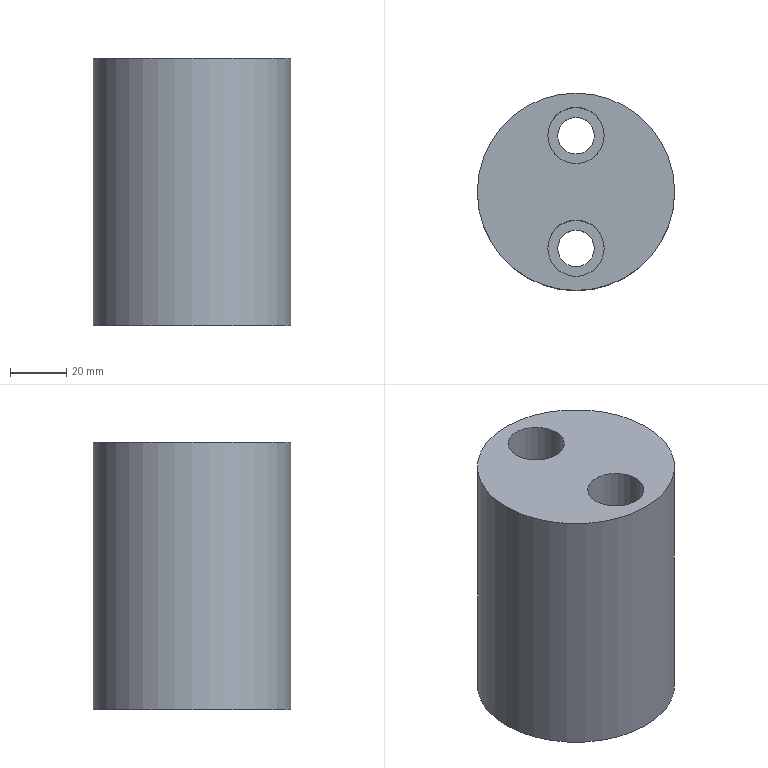Part | NX | features solid 2 | 1 solid | 9 faces | box 70 x 70 x 95 mm | volume 316798 mm3 | cylinder 5 | plane 4 | commonest cylinder face diameters 13 x2 20 x2 70 x1
STEP:
#1=CARTESIAN_POINT('',(-354.,-240.,110.));
#2=VERTEX_POINT('',#1);
#3=CARTESIAN_POINT('',(-389.,-240.,110.));
#4=DIRECTION('',(0.,0.,1.));
#5=DIRECTION('',(1.,0.,0.));
#6=AXIS2_PLACEMENT_3D('',#3,#4,#5);
#7=CIRCLE('',#6,35.);
#8=EDGE_CURVE('',#2,#2,#7,.T.);
#9=ORIENTED_EDGE('',*,*,#8,.T.);
#10=EDGE_LOOP('',(#9));
#11=FACE_BOUND('',#10,.T.);
#12=CARTESIAN_POINT('',(-354.,-240.,205.));
#13=VERTEX_POINT('',#12);
#14=CARTESIAN_POINT('',(-389.,-240.,205.));
#15=DIRECTION('',(0.,0.,1.));
#16=DIRECTION('',(1.,0.,0.));
#17=AXIS2_PLACEMENT_3D('',#14,#15,#16);
#18=CIRCLE('',#17,35.);
#19=EDGE_CURVE('',#13,#13,#18,.T.);
#20=ORIENTED_EDGE('',*,*,#19,.F.);
#21=EDGE_LOOP('',(#20));
#22=FACE_BOUND('',#21,.T.);
#23=CARTESIAN_POINT('',(-389.,-240.,-95.));
#24=DIRECTION('',(0.,0.,1.));
#25=DIRECTION('',(1.,0.,0.));
#26=AXIS2_PLACEMENT_3D('',#23,#24,#25);
#27=CYLINDRICAL_SURFACE('',#26,35.);
#28=ADVANCED_FACE('',(#11,#22),#27,.T.);
#29=CARTESIAN_POINT('',(-382.5,-220.,110.));
#30=VERTEX_POINT('',#29);
#31=CARTESIAN_POINT('',(-389.,-220.,110.));
#32=DIRECTION('',(0.,0.,1.));
#33=DIRECTION('',(1.,0.,0.));
#34=AXIS2_PLACEMENT_3D('',#31,#32,#33);
#35=CIRCLE('',#34,6.5);
#36=EDGE_CURVE('',#30,#30,#35,.T.);
#37=ORIENTED_EDGE('',*,*,#36,.T.);
#38=EDGE_LOOP('',(#37));
#39=FACE_BOUND('',#38,.T.);
#40=CARTESIAN_POINT('',(-382.5,-260.,110.));
#41=VERTEX_POINT('',#40);
#42=CARTESIAN_POINT('',(-389.,-260.,110.));
#43=DIRECTION('',(0.,0.,1.));
#44=DIRECTION('',(1.,0.,0.));
#45=AXIS2_PLACEMENT_3D('',#42,#43,#44);
#46=CIRCLE('',#45,6.5);
#47=EDGE_CURVE('',#41,#41,#46,.T.);
#48=ORIENTED_EDGE('',*,*,#47,.T.);
#49=EDGE_LOOP('',(#48));
#50=FACE_BOUND('',#49,.T.);
#51=ORIENTED_EDGE('',*,*,#8,.F.);
#52=EDGE_LOOP('',(#51));
#53=FACE_BOUND('',#52,.T.);
#54=CARTESIAN_POINT('',(-389.,-240.,110.));
#55=DIRECTION('',(0.,0.,1.));
#56=DIRECTION('',(1.,0.,0.));
#57=AXIS2_PLACEMENT_3D('',#54,#55,#56);
#58=PLANE('',#57);
#59=ADVANCED_FACE('',(#39,#50,#53),#58,.F.);
#60=CARTESIAN_POINT('',(-379.,-220.,205.));
#61=VERTEX_POINT('',#60);
#62=CARTESIAN_POINT('',(-389.,-220.,205.));
#63=DIRECTION('',(0.,0.,1.));
#64=DIRECTION('',(1.,0.,0.));
#65=AXIS2_PLACEMENT_3D('',#62,#63,#64);
#66=CIRCLE('',#65,10.);
#67=EDGE_CURVE('',#61,#61,#66,.T.);
#68=ORIENTED_EDGE('',*,*,#67,.F.);
#69=EDGE_LOOP('',(#68));
#70=FACE_BOUND('',#69,.T.);
#71=CARTESIAN_POINT('',(-379.,-260.,205.));
#72=VERTEX_POINT('',#71);
#73=CARTESIAN_POINT('',(-389.,-260.,205.));
#74=DIRECTION('',(0.,0.,1.));
#75=DIRECTION('',(1.,0.,0.));
#76=AXIS2_PLACEMENT_3D('',#73,#74,#75);
#77=CIRCLE('',#76,10.);
#78=EDGE_CURVE('',#72,#72,#77,.T.);
#79=ORIENTED_EDGE('',*,*,#78,.F.);
#80=EDGE_LOOP('',(#79));
#81=FACE_BOUND('',#80,.T.);
#82=ORIENTED_EDGE('',*,*,#19,.T.);
#83=EDGE_LOOP('',(#82));
#84=FACE_BOUND('',#83,.T.);
#85=CARTESIAN_POINT('',(-389.,-240.,205.));
#86=DIRECTION('',(0.,0.,1.));
#87=DIRECTION('',(1.,0.,0.));
#88=AXIS2_PLACEMENT_3D('',#85,#86,#87);
#89=PLANE('',#88);
#90=ADVANCED_FACE('',(#70,#81,#84),#89,.T.);
#91=CARTESIAN_POINT('',(-395.5,-260.,140.));
#92=VERTEX_POINT('',#91);
#93=CARTESIAN_POINT('',(-389.,-260.,140.));
#94=DIRECTION('',(0.,0.,-1.));
#95=DIRECTION('',(-1.,0.,0.));
#96=AXIS2_PLACEMENT_3D('',#93,#94,#95);
#97=CIRCLE('',#96,6.5);
#98=EDGE_CURVE('',#92,#92,#97,.F.);
#99=ORIENTED_EDGE('',*,*,#98,.T.);
#100=EDGE_LOOP('',(#99));
#101=FACE_BOUND('',#100,.T.);
#102=ORIENTED_EDGE('',*,*,#47,.F.);
#103=EDGE_LOOP('',(#102));
#104=FACE_BOUND('',#103,.T.);
#105=CARTESIAN_POINT('',(-389.,-260.,80.));
#106=DIRECTION('',(0.,0.,1.));
#107=DIRECTION('',(1.,0.,0.));
#108=AXIS2_PLACEMENT_3D('',#105,#106,#107);
#109=CYLINDRICAL_SURFACE('',#108,6.5);
#110=ADVANCED_FACE('',(#101,#104),#109,.F.);
#111=ORIENTED_EDGE('',*,*,#98,.F.);
#112=EDGE_LOOP('',(#111));
#113=FACE_BOUND('',#112,.T.);
#114=CARTESIAN_POINT('',(-379.,-260.,140.));
#115=VERTEX_POINT('',#114);
#116=CARTESIAN_POINT('',(-389.,-260.,140.));
#117=DIRECTION('',(0.,0.,1.));
#118=DIRECTION('',(1.,0.,0.));
#119=AXIS2_PLACEMENT_3D('',#116,#117,#118);
#120=CIRCLE('',#119,10.);
#121=EDGE_CURVE('',#115,#115,#120,.T.);
#122=ORIENTED_EDGE('',*,*,#121,.T.);
#123=EDGE_LOOP('',(#122));
#124=FACE_BOUND('',#123,.T.);
#125=CARTESIAN_POINT('',(-389.,-260.,140.));
#126=DIRECTION('',(0.,0.,-1.));
#127=DIRECTION('',(-1.,0.,0.));
#128=AXIS2_PLACEMENT_3D('',#125,#126,#127);
#129=PLANE('',#128);
#130=ADVANCED_FACE('',(#113,#124),#129,.F.);
#131=ORIENTED_EDGE('',*,*,#78,.T.);
#132=EDGE_LOOP('',(#131));
#133=FACE_BOUND('',#132,.T.);
#134=ORIENTED_EDGE('',*,*,#121,.F.);
#135=EDGE_LOOP('',(#134));
#136=FACE_BOUND('',#135,.T.);
#137=CARTESIAN_POINT('',(-389.,-260.,140.));
#138=DIRECTION('',(0.,0.,1.));
#139=DIRECTION('',(1.,0.,0.));
#140=AXIS2_PLACEMENT_3D('',#137,#138,#139);
#141=CYLINDRICAL_SURFACE('',#140,10.);
#142=ADVANCED_FACE('',(#133,#136),#141,.F.);
#143=CARTESIAN_POINT('',(-395.5,-220.,140.));
#144=VERTEX_POINT('',#143);
#145=CARTESIAN_POINT('',(-389.,-220.,140.));
#146=DIRECTION('',(0.,0.,-1.));
#147=DIRECTION('',(-1.,0.,0.));
#148=AXIS2_PLACEMENT_3D('',#145,#146,#147);
#149=CIRCLE('',#148,6.5);
#150=EDGE_CURVE('',#144,#144,#149,.F.);
#151=ORIENTED_EDGE('',*,*,#150,.T.);
#152=EDGE_LOOP('',(#151));
#153=FACE_BOUND('',#152,.T.);
#154=ORIENTED_EDGE('',*,*,#36,.F.);
#155=EDGE_LOOP('',(#154));
#156=FACE_BOUND('',#155,.T.);
#157=CARTESIAN_POINT('',(-389.,-220.,80.));
#158=DIRECTION('',(0.,0.,1.));
#159=DIRECTION('',(1.,0.,0.));
#160=AXIS2_PLACEMENT_3D('',#157,#158,#159);
#161=CYLINDRICAL_SURFACE('',#160,6.5);
#162=ADVANCED_FACE('',(#153,#156),#161,.F.);
#163=ORIENTED_EDGE('',*,*,#150,.F.);
#164=EDGE_LOOP('',(#163));
#165=FACE_BOUND('',#164,.T.);
#166=CARTESIAN_POINT('',(-379.,-220.,140.));
#167=VERTEX_POINT('',#166);
#168=CARTESIAN_POINT('',(-389.,-220.,140.));
#169=DIRECTION('',(0.,0.,1.));
#170=DIRECTION('',(1.,0.,0.));
#171=AXIS2_PLACEMENT_3D('',#168,#169,#170);
#172=CIRCLE('',#171,10.);
#173=EDGE_CURVE('',#167,#167,#172,.T.);
#174=ORIENTED_EDGE('',*,*,#173,.T.);
#175=EDGE_LOOP('',(#174));
#176=FACE_BOUND('',#175,.T.);
#177=CARTESIAN_POINT('',(-389.,-220.,140.));
#178=DIRECTION('',(0.,0.,-1.));
#179=DIRECTION('',(-1.,0.,0.));
#180=AXIS2_PLACEMENT_3D('',#177,#178,#179);
#181=PLANE('',#180);
#182=ADVANCED_FACE('',(#165,#176),#181,.F.);
#183=ORIENTED_EDGE('',*,*,#67,.T.);
#184=EDGE_LOOP('',(#183));
#185=FACE_BOUND('',#184,.T.);
#186=ORIENTED_EDGE('',*,*,#173,.F.);
#187=EDGE_LOOP('',(#186));
#188=FACE_BOUND('',#187,.T.);
#189=CARTESIAN_POINT('',(-389.,-220.,140.));
#190=DIRECTION('',(0.,0.,1.));
#191=DIRECTION('',(1.,0.,0.));
#192=AXIS2_PLACEMENT_3D('',#189,#190,#191);
#193=CYLINDRICAL_SURFACE('',#192,10.);
#194=ADVANCED_FACE('',(#185,#188),#193,.F.);
#195=CLOSED_SHELL('',(#28,#59,#90,#110,#130,#142,#162,#182,#194));
#196=MANIFOLD_SOLID_BREP('',#195);
#197=(LENGTH_UNIT()NAMED_UNIT(*)SI_UNIT(.MILLI.,.METRE.));
#198=UNCERTAINTY_MEASURE_WITH_UNIT(LENGTH_MEASURE(0.00001),#197,'','');
#199=(NAMED_UNIT(*)PLANE_ANGLE_UNIT()SI_UNIT($,.RADIAN.));
#200=(NAMED_UNIT(*)SI_UNIT($,.STERADIAN.)SOLID_ANGLE_UNIT());
#201=(GEOMETRIC_REPRESENTATION_CONTEXT(3)GLOBAL_UNCERTAINTY_ASSIGNED_CONTEXT((#198))GLOBAL_UNIT_ASSIGNED_CONTEXT((#197,#199,#200))REPRESENTATION_CONTEXT('',''));
#202=ADVANCED_BREP_SHAPE_REPRESENTATION('',(#196),#201);